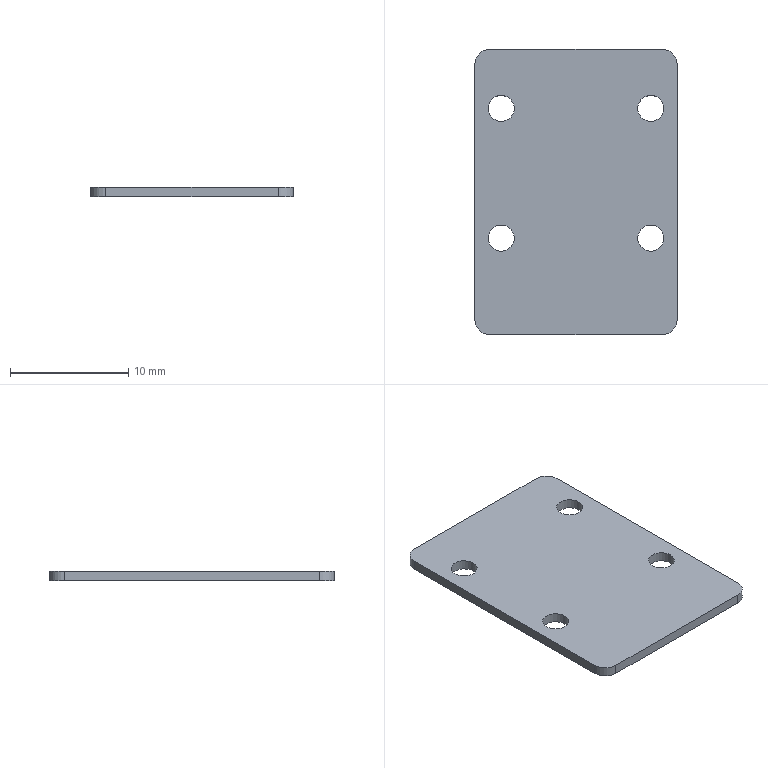Part | STEP file | VSWR protection V+PCB | 1 solid | 14 faces | box 17.08 x 24.07 x 0.832 mm | volume 328.245 mm3 | cylinder 8 | plane 6 | commonest cylinder face diameters 2.2 x4 2.54 x4
STEP:
#1=CARTESIAN_POINT('',(0.,0.,0.));
#2=DIRECTION('',(0.,0.,1.));
#3=DIRECTION('',(1.,0.,0.));
#4=AXIS2_PLACEMENT_3D('',#1,#2,#3);
#5=CARTESIAN_POINT('',(74.34,77.234,-0.832));
#6=VERTEX_POINT('',#5);
#7=CARTESIAN_POINT('',(73.24,77.234,-0.832));
#8=DIRECTION('',(0.,0.,1.));
#9=DIRECTION('',(1.,0.,0.));
#10=AXIS2_PLACEMENT_3D('',#7,#8,#9);
#11=CIRCLE('',#10,1.1);
#12=CARTESIAN_POINT('',(72.28,70.364,-0.832));
#13=DIRECTION('',(0.,0.,1.));
#14=DIRECTION('',(1.,0.,0.));
#15=AXIS2_PLACEMENT_3D('',#12,#13,#14);
#16=PLANE('',#15);
#17=CARTESIAN_POINT('',(0.96,6.87));
#18=DIRECTION('',(1.,0.));
#19=AXIS2_PLACEMENT_2D('',#17,#18);
#20=CIRCLE('',#19,1.1);
#21=(GEOMETRIC_REPRESENTATION_CONTEXT(2)PARAMETRIC_REPRESENTATION_CONTEXT()REPRESENTATION_CONTEXT('',''));
#22=DEFINITIONAL_REPRESENTATION('',(#20),#21);
#23=PCURVE('',#16,#22);
#24=CARTESIAN_POINT('',(73.24,77.234,-0.832));
#25=DIRECTION('',(0.,0.,1.));
#26=DIRECTION('',(1.,0.,0.));
#27=AXIS2_PLACEMENT_3D('',#24,#25,#26);
#28=CYLINDRICAL_SURFACE('',#27,1.1);
#29=CARTESIAN_POINT('',(0.,0.));
#30=DIRECTION('',(1.,0.));
#31=VECTOR('',#30,1.);
#32=LINE('',#29,#31);
#33=(GEOMETRIC_REPRESENTATION_CONTEXT(2)PARAMETRIC_REPRESENTATION_CONTEXT()REPRESENTATION_CONTEXT('',''));
#34=DEFINITIONAL_REPRESENTATION('',(#32),#33);
#35=PCURVE('',#28,#34);
#36=SURFACE_CURVE('',#11,(#23,#35),.PCURVE_S1.);
#37=EDGE_CURVE('',#6,#6,#36,.T.);
#38=ORIENTED_EDGE('',*,*,#37,.T.);
#39=EDGE_LOOP('',(#38));
#40=FACE_BOUND('',#39,.T.);
#41=CARTESIAN_POINT('',(86.96,77.234,-0.832));
#42=VERTEX_POINT('',#41);
#43=CARTESIAN_POINT('',(85.86,77.234,-0.832));
#44=DIRECTION('',(0.,0.,1.));
#45=DIRECTION('',(1.,0.,0.));
#46=AXIS2_PLACEMENT_3D('',#43,#44,#45);
#47=CIRCLE('',#46,1.1);
#48=CARTESIAN_POINT('',(13.58,6.87));
#49=DIRECTION('',(1.,0.));
#50=AXIS2_PLACEMENT_2D('',#48,#49);
#51=CIRCLE('',#50,1.1);
#52=(GEOMETRIC_REPRESENTATION_CONTEXT(2)PARAMETRIC_REPRESENTATION_CONTEXT()REPRESENTATION_CONTEXT('',''));
#53=DEFINITIONAL_REPRESENTATION('',(#51),#52);
#54=PCURVE('',#16,#53);
#55=CARTESIAN_POINT('',(85.86,77.234,-0.832));
#56=DIRECTION('',(0.,0.,1.));
#57=DIRECTION('',(1.,0.,0.));
#58=AXIS2_PLACEMENT_3D('',#55,#56,#57);
#59=CYLINDRICAL_SURFACE('',#58,1.1);
#60=CARTESIAN_POINT('',(0.,0.));
#61=DIRECTION('',(1.,0.));
#62=VECTOR('',#61,1.);
#63=LINE('',#60,#62);
#64=(GEOMETRIC_REPRESENTATION_CONTEXT(2)PARAMETRIC_REPRESENTATION_CONTEXT()REPRESENTATION_CONTEXT('',''));
#65=DEFINITIONAL_REPRESENTATION('',(#63),#64);
#66=PCURVE('',#59,#65);
#67=SURFACE_CURVE('',#47,(#54,#66),.PCURVE_S1.);
#68=EDGE_CURVE('',#42,#42,#67,.T.);
#69=ORIENTED_EDGE('',*,*,#68,.T.);
#70=EDGE_LOOP('',(#69));
#71=FACE_BOUND('',#70,.T.);
#72=CARTESIAN_POINT('',(86.96,88.184,-0.832));
#73=VERTEX_POINT('',#72);
#74=CARTESIAN_POINT('',(85.86,88.184,-0.832));
#75=DIRECTION('',(0.,0.,1.));
#76=DIRECTION('',(1.,0.,0.));
#77=AXIS2_PLACEMENT_3D('',#74,#75,#76);
#78=CIRCLE('',#77,1.1);
#79=CARTESIAN_POINT('',(13.58,17.82));
#80=DIRECTION('',(1.,0.));
#81=AXIS2_PLACEMENT_2D('',#79,#80);
#82=CIRCLE('',#81,1.1);
#83=(GEOMETRIC_REPRESENTATION_CONTEXT(2)PARAMETRIC_REPRESENTATION_CONTEXT()REPRESENTATION_CONTEXT('',''));
#84=DEFINITIONAL_REPRESENTATION('',(#82),#83);
#85=PCURVE('',#16,#84);
#86=CARTESIAN_POINT('',(85.86,88.184,-0.832));
#87=DIRECTION('',(0.,0.,1.));
#88=DIRECTION('',(1.,0.,0.));
#89=AXIS2_PLACEMENT_3D('',#86,#87,#88);
#90=CYLINDRICAL_SURFACE('',#89,1.1);
#91=CARTESIAN_POINT('',(0.,0.));
#92=DIRECTION('',(1.,0.));
#93=VECTOR('',#92,1.);
#94=LINE('',#91,#93);
#95=(GEOMETRIC_REPRESENTATION_CONTEXT(2)PARAMETRIC_REPRESENTATION_CONTEXT()REPRESENTATION_CONTEXT('',''));
#96=DEFINITIONAL_REPRESENTATION('',(#94),#95);
#97=PCURVE('',#90,#96);
#98=SURFACE_CURVE('',#78,(#85,#97),.PCURVE_S1.);
#99=EDGE_CURVE('',#73,#73,#98,.T.);
#100=ORIENTED_EDGE('',*,*,#99,.T.);
#101=EDGE_LOOP('',(#100));
#102=FACE_BOUND('',#101,.T.);
#103=CARTESIAN_POINT('',(71.01,91.894,-0.832));
#104=VERTEX_POINT('',#103);
#105=CARTESIAN_POINT('',(71.01,70.364,-0.832));
#106=VERTEX_POINT('',#105);
#107=CARTESIAN_POINT('',(71.01,91.894,-0.832));
#108=DIRECTION('',(0.,-1.,0.));
#109=VECTOR('',#108,1.);
#110=LINE('',#107,#109);
#111=CARTESIAN_POINT('',(-1.27,21.53));
#112=DIRECTION('',(0.,-1.));
#113=VECTOR('',#112,1.);
#114=LINE('',#111,#113);
#115=(GEOMETRIC_REPRESENTATION_CONTEXT(2)PARAMETRIC_REPRESENTATION_CONTEXT()REPRESENTATION_CONTEXT('',''));
#116=DEFINITIONAL_REPRESENTATION('',(#114),#115);
#117=PCURVE('',#16,#116);
#118=CARTESIAN_POINT('',(71.01,91.894,-0.832));
#119=DIRECTION('',(-1.,0.,0.));
#120=DIRECTION('',(0.,0.,1.));
#121=AXIS2_PLACEMENT_3D('',#118,#119,#120);
#122=PLANE('',#121);
#123=CARTESIAN_POINT('',(0.,0.));
#124=DIRECTION('',(0.,-1.));
#125=VECTOR('',#124,1.);
#126=LINE('',#123,#125);
#127=(GEOMETRIC_REPRESENTATION_CONTEXT(2)PARAMETRIC_REPRESENTATION_CONTEXT()REPRESENTATION_CONTEXT('',''));
#128=DEFINITIONAL_REPRESENTATION('',(#126),#127);
#129=PCURVE('',#122,#128);
#130=SURFACE_CURVE('',#110,(#117,#129),.PCURVE_S1.);
#131=EDGE_CURVE('',#104,#106,#130,.T.);
#132=ORIENTED_EDGE('',*,*,#131,.F.);
#133=CARTESIAN_POINT('',(72.28,93.164,-0.832));
#134=VERTEX_POINT('',#133);
#135=CARTESIAN_POINT('',(72.28,91.894,-0.832));
#136=DIRECTION('',(0.,0.,1.));
#137=DIRECTION('',(1.,0.,0.));
#138=AXIS2_PLACEMENT_3D('',#135,#136,#137);
#139=CIRCLE('',#138,1.27);
#140=CARTESIAN_POINT('',(0.,21.53));
#141=DIRECTION('',(1.,0.));
#142=AXIS2_PLACEMENT_2D('',#140,#141);
#143=CIRCLE('',#142,1.27);
#144=(GEOMETRIC_REPRESENTATION_CONTEXT(2)PARAMETRIC_REPRESENTATION_CONTEXT()REPRESENTATION_CONTEXT('',''));
#145=DEFINITIONAL_REPRESENTATION('',(#143),#144);
#146=PCURVE('',#16,#145);
#147=CARTESIAN_POINT('',(72.28,91.894,-0.832));
#148=DIRECTION('',(0.,0.,1.));
#149=DIRECTION('',(1.,0.,0.));
#150=AXIS2_PLACEMENT_3D('',#147,#148,#149);
#151=CYLINDRICAL_SURFACE('',#150,1.27);
#152=CARTESIAN_POINT('',(0.,0.));
#153=DIRECTION('',(1.,0.));
#154=VECTOR('',#153,1.);
#155=LINE('',#152,#154);
#156=(GEOMETRIC_REPRESENTATION_CONTEXT(2)PARAMETRIC_REPRESENTATION_CONTEXT()REPRESENTATION_CONTEXT('',''));
#157=DEFINITIONAL_REPRESENTATION('',(#155),#156);
#158=PCURVE('',#151,#157);
#159=SURFACE_CURVE('',#139,(#146,#158),.PCURVE_S1.);
#160=EDGE_CURVE('',#134,#104,#159,.T.);
#161=ORIENTED_EDGE('',*,*,#160,.F.);
#162=CARTESIAN_POINT('',(86.82,93.164,-0.832));
#163=VERTEX_POINT('',#162);
#164=CARTESIAN_POINT('',(86.82,93.164,-0.832));
#165=DIRECTION('',(-1.,0.,0.));
#166=VECTOR('',#165,1.);
#167=LINE('',#164,#166);
#168=CARTESIAN_POINT('',(14.54,22.8));
#169=DIRECTION('',(-1.,0.));
#170=VECTOR('',#169,1.);
#171=LINE('',#168,#170);
#172=(GEOMETRIC_REPRESENTATION_CONTEXT(2)PARAMETRIC_REPRESENTATION_CONTEXT()REPRESENTATION_CONTEXT('',''));
#173=DEFINITIONAL_REPRESENTATION('',(#171),#172);
#174=PCURVE('',#16,#173);
#175=CARTESIAN_POINT('',(79.55,93.164,-0.832));
#176=DIRECTION('',(0.,1.,0.));
#177=DIRECTION('',(0.,0.,1.));
#178=AXIS2_PLACEMENT_3D('',#175,#176,#177);
#179=PLANE('',#178);
#180=CARTESIAN_POINT('',(0.,7.27));
#181=DIRECTION('',(0.,-1.));
#182=VECTOR('',#181,1.);
#183=LINE('',#180,#182);
#184=(GEOMETRIC_REPRESENTATION_CONTEXT(2)PARAMETRIC_REPRESENTATION_CONTEXT()REPRESENTATION_CONTEXT('',''));
#185=DEFINITIONAL_REPRESENTATION('',(#183),#184);
#186=PCURVE('',#179,#185);
#187=SURFACE_CURVE('',#167,(#174,#186),.PCURVE_S1.);
#188=EDGE_CURVE('',#163,#134,#187,.T.);
#189=ORIENTED_EDGE('',*,*,#188,.F.);
#190=CARTESIAN_POINT('',(88.09,91.894,-0.832));
#191=VERTEX_POINT('',#190);
#192=CARTESIAN_POINT('',(86.82,91.894,-0.832));
#193=DIRECTION('',(0.,0.,1.));
#194=DIRECTION('',(1.,0.,0.));
#195=AXIS2_PLACEMENT_3D('',#192,#193,#194);
#196=CIRCLE('',#195,1.27);
#197=CARTESIAN_POINT('',(14.54,21.53));
#198=DIRECTION('',(1.,0.));
#199=AXIS2_PLACEMENT_2D('',#197,#198);
#200=CIRCLE('',#199,1.27);
#201=(GEOMETRIC_REPRESENTATION_CONTEXT(2)PARAMETRIC_REPRESENTATION_CONTEXT()REPRESENTATION_CONTEXT('',''));
#202=DEFINITIONAL_REPRESENTATION('',(#200),#201);
#203=PCURVE('',#16,#202);
#204=CARTESIAN_POINT('',(86.82,91.894,-0.832));
#205=DIRECTION('',(0.,0.,1.));
#206=DIRECTION('',(1.,0.,0.));
#207=AXIS2_PLACEMENT_3D('',#204,#205,#206);
#208=CYLINDRICAL_SURFACE('',#207,1.27);
#209=CARTESIAN_POINT('',(0.,0.));
#210=DIRECTION('',(1.,0.));
#211=VECTOR('',#210,1.);
#212=LINE('',#209,#211);
#213=(GEOMETRIC_REPRESENTATION_CONTEXT(2)PARAMETRIC_REPRESENTATION_CONTEXT()REPRESENTATION_CONTEXT('',''));
#214=DEFINITIONAL_REPRESENTATION('',(#212),#213);
#215=PCURVE('',#208,#214);
#216=SURFACE_CURVE('',#196,(#203,#215),.PCURVE_S1.);
#217=EDGE_CURVE('',#191,#163,#216,.T.);
#218=ORIENTED_EDGE('',*,*,#217,.F.);
#219=CARTESIAN_POINT('',(88.09,70.364,-0.832));
#220=VERTEX_POINT('',#219);
#221=CARTESIAN_POINT('',(88.09,70.364,-0.832));
#222=DIRECTION('',(0.,1.,0.));
#223=VECTOR('',#222,1.);
#224=LINE('',#221,#223);
#225=CARTESIAN_POINT('',(15.81,0.));
#226=DIRECTION('',(0.,1.));
#227=VECTOR('',#226,1.);
#228=LINE('',#225,#227);
#229=(GEOMETRIC_REPRESENTATION_CONTEXT(2)PARAMETRIC_REPRESENTATION_CONTEXT()REPRESENTATION_CONTEXT('',''));
#230=DEFINITIONAL_REPRESENTATION('',(#228),#229);
#231=PCURVE('',#16,#230);
#232=CARTESIAN_POINT('',(88.09,70.364,-0.832));
#233=DIRECTION('',(1.,0.,0.));
#234=DIRECTION('',(0.,0.,-1.));
#235=AXIS2_PLACEMENT_3D('',#232,#233,#234);
#236=PLANE('',#235);
#237=CARTESIAN_POINT('',(0.,0.));
#238=DIRECTION('',(0.,1.));
#239=VECTOR('',#238,1.);
#240=LINE('',#237,#239);
#241=(GEOMETRIC_REPRESENTATION_CONTEXT(2)PARAMETRIC_REPRESENTATION_CONTEXT()REPRESENTATION_CONTEXT('',''));
#242=DEFINITIONAL_REPRESENTATION('',(#240),#241);
#243=PCURVE('',#236,#242);
#244=SURFACE_CURVE('',#224,(#231,#243),.PCURVE_S1.);
#245=EDGE_CURVE('',#220,#191,#244,.T.);
#246=ORIENTED_EDGE('',*,*,#245,.F.);
#247=CARTESIAN_POINT('',(86.82,69.094,-0.832));
#248=VERTEX_POINT('',#247);
#249=CARTESIAN_POINT('',(86.82,70.364,-0.832));
#250=DIRECTION('',(0.,0.,1.));
#251=DIRECTION('',(1.,0.,0.));
#252=AXIS2_PLACEMENT_3D('',#249,#250,#251);
#253=CIRCLE('',#252,1.27);
#254=CARTESIAN_POINT('',(14.54,0.));
#255=DIRECTION('',(1.,0.));
#256=AXIS2_PLACEMENT_2D('',#254,#255);
#257=CIRCLE('',#256,1.27);
#258=(GEOMETRIC_REPRESENTATION_CONTEXT(2)PARAMETRIC_REPRESENTATION_CONTEXT()REPRESENTATION_CONTEXT('',''));
#259=DEFINITIONAL_REPRESENTATION('',(#257),#258);
#260=PCURVE('',#16,#259);
#261=CARTESIAN_POINT('',(86.82,70.364,-0.832));
#262=DIRECTION('',(0.,0.,1.));
#263=DIRECTION('',(1.,0.,0.));
#264=AXIS2_PLACEMENT_3D('',#261,#262,#263);
#265=CYLINDRICAL_SURFACE('',#264,1.27);
#266=CARTESIAN_POINT('',(0.,0.));
#267=DIRECTION('',(1.,0.));
#268=VECTOR('',#267,1.);
#269=LINE('',#266,#268);
#270=(GEOMETRIC_REPRESENTATION_CONTEXT(2)PARAMETRIC_REPRESENTATION_CONTEXT()REPRESENTATION_CONTEXT('',''));
#271=DEFINITIONAL_REPRESENTATION('',(#269),#270);
#272=PCURVE('',#265,#271);
#273=SURFACE_CURVE('',#253,(#260,#272),.PCURVE_S1.);
#274=EDGE_CURVE('',#248,#220,#273,.T.);
#275=ORIENTED_EDGE('',*,*,#274,.F.);
#276=CARTESIAN_POINT('',(72.28,69.094,-0.832));
#277=VERTEX_POINT('',#276);
#278=CARTESIAN_POINT('',(72.28,69.094,-0.832));
#279=DIRECTION('',(1.,0.,0.));
#280=VECTOR('',#279,1.);
#281=LINE('',#278,#280);
#282=CARTESIAN_POINT('',(0.,-1.27));
#283=DIRECTION('',(1.,0.));
#284=VECTOR('',#283,1.);
#285=LINE('',#282,#284);
#286=(GEOMETRIC_REPRESENTATION_CONTEXT(2)PARAMETRIC_REPRESENTATION_CONTEXT()REPRESENTATION_CONTEXT('',''));
#287=DEFINITIONAL_REPRESENTATION('',(#285),#286);
#288=PCURVE('',#16,#287);
#289=CARTESIAN_POINT('',(72.28,69.094,-0.832));
#290=DIRECTION('',(0.,-1.,0.));
#291=DIRECTION('',(0.,0.,-1.));
#292=AXIS2_PLACEMENT_3D('',#289,#290,#291);
#293=PLANE('',#292);
#294=CARTESIAN_POINT('',(0.,0.));
#295=DIRECTION('',(0.,1.));
#296=VECTOR('',#295,1.);
#297=LINE('',#294,#296);
#298=(GEOMETRIC_REPRESENTATION_CONTEXT(2)PARAMETRIC_REPRESENTATION_CONTEXT()REPRESENTATION_CONTEXT('',''));
#299=DEFINITIONAL_REPRESENTATION('',(#297),#298);
#300=PCURVE('',#293,#299);
#301=SURFACE_CURVE('',#281,(#288,#300),.PCURVE_S1.);
#302=EDGE_CURVE('',#277,#248,#301,.T.);
#303=ORIENTED_EDGE('',*,*,#302,.F.);
#304=CARTESIAN_POINT('',(72.28,70.364,-0.832));
#305=DIRECTION('',(0.,0.,1.));
#306=DIRECTION('',(1.,0.,0.));
#307=AXIS2_PLACEMENT_3D('',#304,#305,#306);
#308=CIRCLE('',#307,1.27);
#309=CARTESIAN_POINT('',(0.,0.));
#310=DIRECTION('',(1.,0.));
#311=AXIS2_PLACEMENT_2D('',#309,#310);
#312=CIRCLE('',#311,1.27);
#313=(GEOMETRIC_REPRESENTATION_CONTEXT(2)PARAMETRIC_REPRESENTATION_CONTEXT()REPRESENTATION_CONTEXT('',''));
#314=DEFINITIONAL_REPRESENTATION('',(#312),#313);
#315=PCURVE('',#16,#314);
#316=CARTESIAN_POINT('',(72.28,70.364,-0.832));
#317=DIRECTION('',(0.,0.,1.));
#318=DIRECTION('',(1.,0.,0.));
#319=AXIS2_PLACEMENT_3D('',#316,#317,#318);
#320=CYLINDRICAL_SURFACE('',#319,1.27);
#321=CARTESIAN_POINT('',(0.,0.));
#322=DIRECTION('',(1.,0.));
#323=VECTOR('',#322,1.);
#324=LINE('',#321,#323);
#325=(GEOMETRIC_REPRESENTATION_CONTEXT(2)PARAMETRIC_REPRESENTATION_CONTEXT()REPRESENTATION_CONTEXT('',''));
#326=DEFINITIONAL_REPRESENTATION('',(#324),#325);
#327=PCURVE('',#320,#326);
#328=SURFACE_CURVE('',#308,(#315,#327),.PCURVE_S1.);
#329=EDGE_CURVE('',#106,#277,#328,.T.);
#330=ORIENTED_EDGE('',*,*,#329,.F.);
#331=EDGE_LOOP('',(#132,#161,#189,#218,#246,#275,#303,#330));
#332=FACE_BOUND('',#331,.T.);
#333=CARTESIAN_POINT('',(74.34,88.184,-0.832));
#334=VERTEX_POINT('',#333);
#335=CARTESIAN_POINT('',(73.24,88.184,-0.832));
#336=DIRECTION('',(0.,0.,-1.));
#337=DIRECTION('',(1.,0.,0.));
#338=AXIS2_PLACEMENT_3D('',#335,#336,#337);
#339=CIRCLE('',#338,1.1);
#340=CARTESIAN_POINT('',(2.06,17.82));
#341=CARTESIAN_POINT('',(2.06,15.915));
#342=CARTESIAN_POINT('',(0.41,16.867));
#343=CARTESIAN_POINT('',(-1.24,17.82));
#344=CARTESIAN_POINT('',(0.41,18.773));
#345=CARTESIAN_POINT('',(2.06,19.725));
#346=CARTESIAN_POINT('',(2.06,17.82));
#347=(BOUNDED_CURVE()B_SPLINE_CURVE(2,(#340,#341,#342,#343,#344,#345,#346),.UNSPECIFIED.,.T.,.F.)B_SPLINE_CURVE_WITH_KNOTS((1,2,2,2,2,1),(-2.094,0.,2.094,4.189,6.283,8.378),.UNSPECIFIED.)CURVE()GEOMETRIC_REPRESENTATION_ITEM()RATIONAL_B_SPLINE_CURVE((1.,0.5,1.,0.5,1.,0.5,1.))REPRESENTATION_ITEM(''));
#348=(GEOMETRIC_REPRESENTATION_CONTEXT(2)PARAMETRIC_REPRESENTATION_CONTEXT()REPRESENTATION_CONTEXT('',''));
#349=DEFINITIONAL_REPRESENTATION('',(#347),#348);
#350=PCURVE('',#16,#349);
#351=CARTESIAN_POINT('',(73.24,88.184,-0.832));
#352=DIRECTION('',(0.,0.,1.));
#353=DIRECTION('',(1.,0.,0.));
#354=AXIS2_PLACEMENT_3D('',#351,#352,#353);
#355=CYLINDRICAL_SURFACE('',#354,1.1);
#356=CARTESIAN_POINT('',(6.283,0.));
#357=DIRECTION('',(-1.,0.));
#358=VECTOR('',#357,1.);
#359=LINE('',#356,#358);
#360=(GEOMETRIC_REPRESENTATION_CONTEXT(2)PARAMETRIC_REPRESENTATION_CONTEXT()REPRESENTATION_CONTEXT('',''));
#361=DEFINITIONAL_REPRESENTATION('',(#359),#360);
#362=PCURVE('',#355,#361);
#363=SURFACE_CURVE('',#339,(#350,#362),.PCURVE_S1.);
#364=EDGE_CURVE('',#334,#334,#363,.T.);
#365=ORIENTED_EDGE('',*,*,#364,.F.);
#366=EDGE_LOOP('',(#365));
#367=FACE_BOUND('',#366,.T.);
#368=ADVANCED_FACE('',(#40,#71,#102,#332,#367),#16,.F.);
#369=CARTESIAN_POINT('',(71.01,91.894,0.));
#370=VERTEX_POINT('',#369);
#371=CARTESIAN_POINT('',(71.01,70.364,0.));
#372=VERTEX_POINT('',#371);
#373=CARTESIAN_POINT('',(71.01,91.894,0.));
#374=DIRECTION('',(0.,-1.,0.));
#375=VECTOR('',#374,1.);
#376=LINE('',#373,#375);
#377=CARTESIAN_POINT('',(72.28,70.364,0.));
#378=DIRECTION('',(0.,0.,1.));
#379=DIRECTION('',(1.,0.,0.));
#380=AXIS2_PLACEMENT_3D('',#377,#378,#379);
#381=PLANE('',#380);
#382=CARTESIAN_POINT('',(-1.27,21.53));
#383=DIRECTION('',(0.,-1.));
#384=VECTOR('',#383,1.);
#385=LINE('',#382,#384);
#386=(GEOMETRIC_REPRESENTATION_CONTEXT(2)PARAMETRIC_REPRESENTATION_CONTEXT()REPRESENTATION_CONTEXT('',''));
#387=DEFINITIONAL_REPRESENTATION('',(#385),#386);
#388=PCURVE('',#381,#387);
#389=CARTESIAN_POINT('',(0.832,0.));
#390=DIRECTION('',(0.,-1.));
#391=VECTOR('',#390,1.);
#392=LINE('',#389,#391);
#393=(GEOMETRIC_REPRESENTATION_CONTEXT(2)PARAMETRIC_REPRESENTATION_CONTEXT()REPRESENTATION_CONTEXT('',''));
#394=DEFINITIONAL_REPRESENTATION('',(#392),#393);
#395=PCURVE('',#122,#394);
#396=SURFACE_CURVE('',#376,(#388,#395),.PCURVE_S1.);
#397=EDGE_CURVE('',#370,#372,#396,.T.);
#398=ORIENTED_EDGE('',*,*,#397,.T.);
#399=CARTESIAN_POINT('',(72.28,69.094,0.));
#400=VERTEX_POINT('',#399);
#401=CARTESIAN_POINT('',(72.28,70.364,0.));
#402=DIRECTION('',(0.,0.,1.));
#403=DIRECTION('',(1.,0.,0.));
#404=AXIS2_PLACEMENT_3D('',#401,#402,#403);
#405=CIRCLE('',#404,1.27);
#406=CARTESIAN_POINT('',(0.,0.));
#407=DIRECTION('',(1.,0.));
#408=AXIS2_PLACEMENT_2D('',#406,#407);
#409=CIRCLE('',#408,1.27);
#410=(GEOMETRIC_REPRESENTATION_CONTEXT(2)PARAMETRIC_REPRESENTATION_CONTEXT()REPRESENTATION_CONTEXT('',''));
#411=DEFINITIONAL_REPRESENTATION('',(#409),#410);
#412=PCURVE('',#381,#411);
#413=CARTESIAN_POINT('',(0.,0.832));
#414=DIRECTION('',(1.,0.));
#415=VECTOR('',#414,1.);
#416=LINE('',#413,#415);
#417=(GEOMETRIC_REPRESENTATION_CONTEXT(2)PARAMETRIC_REPRESENTATION_CONTEXT()REPRESENTATION_CONTEXT('',''));
#418=DEFINITIONAL_REPRESENTATION('',(#416),#417);
#419=PCURVE('',#320,#418);
#420=SURFACE_CURVE('',#405,(#412,#419),.PCURVE_S1.);
#421=EDGE_CURVE('',#372,#400,#420,.T.);
#422=ORIENTED_EDGE('',*,*,#421,.T.);
#423=CARTESIAN_POINT('',(86.82,69.094,0.));
#424=VERTEX_POINT('',#423);
#425=CARTESIAN_POINT('',(72.28,69.094,0.));
#426=DIRECTION('',(1.,0.,0.));
#427=VECTOR('',#426,1.);
#428=LINE('',#425,#427);
#429=CARTESIAN_POINT('',(0.,-1.27));
#430=DIRECTION('',(1.,0.));
#431=VECTOR('',#430,1.);
#432=LINE('',#429,#431);
#433=(GEOMETRIC_REPRESENTATION_CONTEXT(2)PARAMETRIC_REPRESENTATION_CONTEXT()REPRESENTATION_CONTEXT('',''));
#434=DEFINITIONAL_REPRESENTATION('',(#432),#433);
#435=PCURVE('',#381,#434);
#436=CARTESIAN_POINT('',(-0.832,0.));
#437=DIRECTION('',(0.,1.));
#438=VECTOR('',#437,1.);
#439=LINE('',#436,#438);
#440=(GEOMETRIC_REPRESENTATION_CONTEXT(2)PARAMETRIC_REPRESENTATION_CONTEXT()REPRESENTATION_CONTEXT('',''));
#441=DEFINITIONAL_REPRESENTATION('',(#439),#440);
#442=PCURVE('',#293,#441);
#443=SURFACE_CURVE('',#428,(#435,#442),.PCURVE_S1.);
#444=EDGE_CURVE('',#400,#424,#443,.T.);
#445=ORIENTED_EDGE('',*,*,#444,.T.);
#446=CARTESIAN_POINT('',(88.09,70.364,0.));
#447=VERTEX_POINT('',#446);
#448=CARTESIAN_POINT('',(86.82,70.364,0.));
#449=DIRECTION('',(0.,0.,1.));
#450=DIRECTION('',(1.,0.,0.));
#451=AXIS2_PLACEMENT_3D('',#448,#449,#450);
#452=CIRCLE('',#451,1.27);
#453=CARTESIAN_POINT('',(14.54,0.));
#454=DIRECTION('',(1.,0.));
#455=AXIS2_PLACEMENT_2D('',#453,#454);
#456=CIRCLE('',#455,1.27);
#457=(GEOMETRIC_REPRESENTATION_CONTEXT(2)PARAMETRIC_REPRESENTATION_CONTEXT()REPRESENTATION_CONTEXT('',''));
#458=DEFINITIONAL_REPRESENTATION('',(#456),#457);
#459=PCURVE('',#381,#458);
#460=CARTESIAN_POINT('',(0.,0.832));
#461=DIRECTION('',(1.,0.));
#462=VECTOR('',#461,1.);
#463=LINE('',#460,#462);
#464=(GEOMETRIC_REPRESENTATION_CONTEXT(2)PARAMETRIC_REPRESENTATION_CONTEXT()REPRESENTATION_CONTEXT('',''));
#465=DEFINITIONAL_REPRESENTATION('',(#463),#464);
#466=PCURVE('',#265,#465);
#467=SURFACE_CURVE('',#452,(#459,#466),.PCURVE_S1.);
#468=EDGE_CURVE('',#424,#447,#467,.T.);
#469=ORIENTED_EDGE('',*,*,#468,.T.);
#470=CARTESIAN_POINT('',(88.09,91.894,0.));
#471=VERTEX_POINT('',#470);
#472=CARTESIAN_POINT('',(88.09,70.364,0.));
#473=DIRECTION('',(0.,1.,0.));
#474=VECTOR('',#473,1.);
#475=LINE('',#472,#474);
#476=CARTESIAN_POINT('',(15.81,0.));
#477=DIRECTION('',(0.,1.));
#478=VECTOR('',#477,1.);
#479=LINE('',#476,#478);
#480=(GEOMETRIC_REPRESENTATION_CONTEXT(2)PARAMETRIC_REPRESENTATION_CONTEXT()REPRESENTATION_CONTEXT('',''));
#481=DEFINITIONAL_REPRESENTATION('',(#479),#480);
#482=PCURVE('',#381,#481);
#483=CARTESIAN_POINT('',(-0.832,0.));
#484=DIRECTION('',(0.,1.));
#485=VECTOR('',#484,1.);
#486=LINE('',#483,#485);
#487=(GEOMETRIC_REPRESENTATION_CONTEXT(2)PARAMETRIC_REPRESENTATION_CONTEXT()REPRESENTATION_CONTEXT('',''));
#488=DEFINITIONAL_REPRESENTATION('',(#486),#487);
#489=PCURVE('',#236,#488);
#490=SURFACE_CURVE('',#475,(#482,#489),.PCURVE_S1.);
#491=EDGE_CURVE('',#447,#471,#490,.T.);
#492=ORIENTED_EDGE('',*,*,#491,.T.);
#493=CARTESIAN_POINT('',(86.82,93.164,0.));
#494=VERTEX_POINT('',#493);
#495=CARTESIAN_POINT('',(86.82,91.894,0.));
#496=DIRECTION('',(0.,0.,1.));
#497=DIRECTION('',(1.,0.,0.));
#498=AXIS2_PLACEMENT_3D('',#495,#496,#497);
#499=CIRCLE('',#498,1.27);
#500=CARTESIAN_POINT('',(14.54,21.53));
#501=DIRECTION('',(1.,0.));
#502=AXIS2_PLACEMENT_2D('',#500,#501);
#503=CIRCLE('',#502,1.27);
#504=(GEOMETRIC_REPRESENTATION_CONTEXT(2)PARAMETRIC_REPRESENTATION_CONTEXT()REPRESENTATION_CONTEXT('',''));
#505=DEFINITIONAL_REPRESENTATION('',(#503),#504);
#506=PCURVE('',#381,#505);
#507=CARTESIAN_POINT('',(0.,0.832));
#508=DIRECTION('',(1.,0.));
#509=VECTOR('',#508,1.);
#510=LINE('',#507,#509);
#511=(GEOMETRIC_REPRESENTATION_CONTEXT(2)PARAMETRIC_REPRESENTATION_CONTEXT()REPRESENTATION_CONTEXT('',''));
#512=DEFINITIONAL_REPRESENTATION('',(#510),#511);
#513=PCURVE('',#208,#512);
#514=SURFACE_CURVE('',#499,(#506,#513),.PCURVE_S1.);
#515=EDGE_CURVE('',#471,#494,#514,.T.);
#516=ORIENTED_EDGE('',*,*,#515,.T.);
#517=CARTESIAN_POINT('',(72.28,93.164,0.));
#518=VERTEX_POINT('',#517);
#519=CARTESIAN_POINT('',(79.55,93.164,0.));
#520=DIRECTION('',(-1.,0.,0.));
#521=VECTOR('',#520,1.);
#522=LINE('',#519,#521);
#523=CARTESIAN_POINT('',(7.27,22.8));
#524=DIRECTION('',(-1.,0.));
#525=VECTOR('',#524,1.);
#526=LINE('',#523,#525);
#527=(GEOMETRIC_REPRESENTATION_CONTEXT(2)PARAMETRIC_REPRESENTATION_CONTEXT()REPRESENTATION_CONTEXT('',''));
#528=DEFINITIONAL_REPRESENTATION('',(#526),#527);
#529=PCURVE('',#381,#528);
#530=CARTESIAN_POINT('',(0.832,0.));
#531=DIRECTION('',(0.,-1.));
#532=VECTOR('',#531,1.);
#533=LINE('',#530,#532);
#534=(GEOMETRIC_REPRESENTATION_CONTEXT(2)PARAMETRIC_REPRESENTATION_CONTEXT()REPRESENTATION_CONTEXT('',''));
#535=DEFINITIONAL_REPRESENTATION('',(#533),#534);
#536=PCURVE('',#179,#535);
#537=SURFACE_CURVE('',#522,(#529,#536),.PCURVE_S1.);
#538=EDGE_CURVE('',#494,#518,#537,.T.);
#539=ORIENTED_EDGE('',*,*,#538,.T.);
#540=CARTESIAN_POINT('',(72.28,91.894,0.));
#541=DIRECTION('',(0.,0.,1.));
#542=DIRECTION('',(1.,0.,0.));
#543=AXIS2_PLACEMENT_3D('',#540,#541,#542);
#544=CIRCLE('',#543,1.27);
#545=CARTESIAN_POINT('',(0.,21.53));
#546=DIRECTION('',(1.,0.));
#547=AXIS2_PLACEMENT_2D('',#545,#546);
#548=CIRCLE('',#547,1.27);
#549=(GEOMETRIC_REPRESENTATION_CONTEXT(2)PARAMETRIC_REPRESENTATION_CONTEXT()REPRESENTATION_CONTEXT('',''));
#550=DEFINITIONAL_REPRESENTATION('',(#548),#549);
#551=PCURVE('',#381,#550);
#552=CARTESIAN_POINT('',(0.,0.832));
#553=DIRECTION('',(1.,0.));
#554=VECTOR('',#553,1.);
#555=LINE('',#552,#554);
#556=(GEOMETRIC_REPRESENTATION_CONTEXT(2)PARAMETRIC_REPRESENTATION_CONTEXT()REPRESENTATION_CONTEXT('',''));
#557=DEFINITIONAL_REPRESENTATION('',(#555),#556);
#558=PCURVE('',#151,#557);
#559=SURFACE_CURVE('',#544,(#551,#558),.PCURVE_S1.);
#560=EDGE_CURVE('',#518,#370,#559,.T.);
#561=ORIENTED_EDGE('',*,*,#560,.T.);
#562=EDGE_LOOP('',(#398,#422,#445,#469,#492,#516,#539,#561));
#563=FACE_BOUND('',#562,.T.);
#564=CARTESIAN_POINT('',(86.96,88.184,0.));
#565=VERTEX_POINT('',#564);
#566=CARTESIAN_POINT('',(85.86,88.184,0.));
#567=DIRECTION('',(0.,0.,1.));
#568=DIRECTION('',(1.,0.,0.));
#569=AXIS2_PLACEMENT_3D('',#566,#567,#568);
#570=CIRCLE('',#569,1.1);
#571=CARTESIAN_POINT('',(13.58,17.82));
#572=DIRECTION('',(1.,0.));
#573=AXIS2_PLACEMENT_2D('',#571,#572);
#574=CIRCLE('',#573,1.1);
#575=(GEOMETRIC_REPRESENTATION_CONTEXT(2)PARAMETRIC_REPRESENTATION_CONTEXT()REPRESENTATION_CONTEXT('',''));
#576=DEFINITIONAL_REPRESENTATION('',(#574),#575);
#577=PCURVE('',#381,#576);
#578=CARTESIAN_POINT('',(0.,0.832));
#579=DIRECTION('',(1.,0.));
#580=VECTOR('',#579,1.);
#581=LINE('',#578,#580);
#582=(GEOMETRIC_REPRESENTATION_CONTEXT(2)PARAMETRIC_REPRESENTATION_CONTEXT()REPRESENTATION_CONTEXT('',''));
#583=DEFINITIONAL_REPRESENTATION('',(#581),#582);
#584=PCURVE('',#90,#583);
#585=SURFACE_CURVE('',#570,(#577,#584),.PCURVE_S1.);
#586=EDGE_CURVE('',#565,#565,#585,.T.);
#587=ORIENTED_EDGE('',*,*,#586,.F.);
#588=EDGE_LOOP('',(#587));
#589=FACE_BOUND('',#588,.T.);
#590=CARTESIAN_POINT('',(86.96,77.234,0.));
#591=VERTEX_POINT('',#590);
#592=CARTESIAN_POINT('',(85.86,77.234,0.));
#593=DIRECTION('',(0.,0.,1.));
#594=DIRECTION('',(1.,0.,0.));
#595=AXIS2_PLACEMENT_3D('',#592,#593,#594);
#596=CIRCLE('',#595,1.1);
#597=CARTESIAN_POINT('',(13.58,6.87));
#598=DIRECTION('',(1.,0.));
#599=AXIS2_PLACEMENT_2D('',#597,#598);
#600=CIRCLE('',#599,1.1);
#601=(GEOMETRIC_REPRESENTATION_CONTEXT(2)PARAMETRIC_REPRESENTATION_CONTEXT()REPRESENTATION_CONTEXT('',''));
#602=DEFINITIONAL_REPRESENTATION('',(#600),#601);
#603=PCURVE('',#381,#602);
#604=CARTESIAN_POINT('',(0.,0.832));
#605=DIRECTION('',(1.,0.));
#606=VECTOR('',#605,1.);
#607=LINE('',#604,#606);
#608=(GEOMETRIC_REPRESENTATION_CONTEXT(2)PARAMETRIC_REPRESENTATION_CONTEXT()REPRESENTATION_CONTEXT('',''));
#609=DEFINITIONAL_REPRESENTATION('',(#607),#608);
#610=PCURVE('',#59,#609);
#611=SURFACE_CURVE('',#596,(#603,#610),.PCURVE_S1.);
#612=EDGE_CURVE('',#591,#591,#611,.T.);
#613=ORIENTED_EDGE('',*,*,#612,.F.);
#614=EDGE_LOOP('',(#613));
#615=FACE_BOUND('',#614,.T.);
#616=CARTESIAN_POINT('',(74.34,77.234,0.));
#617=VERTEX_POINT('',#616);
#618=CARTESIAN_POINT('',(73.24,77.234,0.));
#619=DIRECTION('',(0.,0.,1.));
#620=DIRECTION('',(1.,0.,0.));
#621=AXIS2_PLACEMENT_3D('',#618,#619,#620);
#622=CIRCLE('',#621,1.1);
#623=CARTESIAN_POINT('',(0.96,6.87));
#624=DIRECTION('',(1.,0.));
#625=AXIS2_PLACEMENT_2D('',#623,#624);
#626=CIRCLE('',#625,1.1);
#627=(GEOMETRIC_REPRESENTATION_CONTEXT(2)PARAMETRIC_REPRESENTATION_CONTEXT()REPRESENTATION_CONTEXT('',''));
#628=DEFINITIONAL_REPRESENTATION('',(#626),#627);
#629=PCURVE('',#381,#628);
#630=CARTESIAN_POINT('',(0.,0.832));
#631=DIRECTION('',(1.,0.));
#632=VECTOR('',#631,1.);
#633=LINE('',#630,#632);
#634=(GEOMETRIC_REPRESENTATION_CONTEXT(2)PARAMETRIC_REPRESENTATION_CONTEXT()REPRESENTATION_CONTEXT('',''));
#635=DEFINITIONAL_REPRESENTATION('',(#633),#634);
#636=PCURVE('',#28,#635);
#637=SURFACE_CURVE('',#622,(#629,#636),.PCURVE_S1.);
#638=EDGE_CURVE('',#617,#617,#637,.T.);
#639=ORIENTED_EDGE('',*,*,#638,.F.);
#640=EDGE_LOOP('',(#639));
#641=FACE_BOUND('',#640,.T.);
#642=CARTESIAN_POINT('',(74.34,88.184,0.));
#643=VERTEX_POINT('',#642);
#644=CARTESIAN_POINT('',(73.24,88.184,0.));
#645=DIRECTION('',(0.,0.,-1.));
#646=DIRECTION('',(1.,0.,0.));
#647=AXIS2_PLACEMENT_3D('',#644,#645,#646);
#648=CIRCLE('',#647,1.1);
#649=CARTESIAN_POINT('',(2.06,17.82));
#650=CARTESIAN_POINT('',(2.06,15.915));
#651=CARTESIAN_POINT('',(0.41,16.867));
#652=CARTESIAN_POINT('',(-1.24,17.82));
#653=CARTESIAN_POINT('',(0.41,18.773));
#654=CARTESIAN_POINT('',(2.06,19.725));
#655=CARTESIAN_POINT('',(2.06,17.82));
#656=(BOUNDED_CURVE()B_SPLINE_CURVE(2,(#649,#650,#651,#652,#653,#654,#655),.UNSPECIFIED.,.T.,.F.)B_SPLINE_CURVE_WITH_KNOTS((1,2,2,2,2,1),(-2.094,0.,2.094,4.189,6.283,8.378),.UNSPECIFIED.)CURVE()GEOMETRIC_REPRESENTATION_ITEM()RATIONAL_B_SPLINE_CURVE((1.,0.5,1.,0.5,1.,0.5,1.))REPRESENTATION_ITEM(''));
#657=(GEOMETRIC_REPRESENTATION_CONTEXT(2)PARAMETRIC_REPRESENTATION_CONTEXT()REPRESENTATION_CONTEXT('',''));
#658=DEFINITIONAL_REPRESENTATION('',(#656),#657);
#659=PCURVE('',#381,#658);
#660=CARTESIAN_POINT('',(6.283,0.832));
#661=DIRECTION('',(-1.,0.));
#662=VECTOR('',#661,1.);
#663=LINE('',#660,#662);
#664=(GEOMETRIC_REPRESENTATION_CONTEXT(2)PARAMETRIC_REPRESENTATION_CONTEXT()REPRESENTATION_CONTEXT('',''));
#665=DEFINITIONAL_REPRESENTATION('',(#663),#664);
#666=PCURVE('',#355,#665);
#667=SURFACE_CURVE('',#648,(#659,#666),.PCURVE_S1.);
#668=EDGE_CURVE('',#643,#643,#667,.T.);
#669=ORIENTED_EDGE('',*,*,#668,.T.);
#670=EDGE_LOOP('',(#669));
#671=FACE_BOUND('',#670,.T.);
#672=ADVANCED_FACE('',(#563,#589,#615,#641,#671),#381,.T.);
#673=ORIENTED_EDGE('',*,*,#397,.F.);
#674=CARTESIAN_POINT('',(71.01,91.894,-0.832));
#675=DIRECTION('',(0.,0.,1.));
#676=VECTOR('',#675,1.);
#677=LINE('',#674,#676);
#678=CARTESIAN_POINT('',(0.,0.));
#679=DIRECTION('',(1.,0.));
#680=VECTOR('',#679,1.);
#681=LINE('',#678,#680);
#682=(GEOMETRIC_REPRESENTATION_CONTEXT(2)PARAMETRIC_REPRESENTATION_CONTEXT()REPRESENTATION_CONTEXT('',''));
#683=DEFINITIONAL_REPRESENTATION('',(#681),#682);
#684=PCURVE('',#122,#683);
#685=CARTESIAN_POINT('',(3.142,0.));
#686=DIRECTION('',(0.,1.));
#687=VECTOR('',#686,1.);
#688=LINE('',#685,#687);
#689=(GEOMETRIC_REPRESENTATION_CONTEXT(2)PARAMETRIC_REPRESENTATION_CONTEXT()REPRESENTATION_CONTEXT('',''));
#690=DEFINITIONAL_REPRESENTATION('',(#688),#689);
#691=PCURVE('',#151,#690);
#692=SURFACE_CURVE('',#677,(#684,#691),.PCURVE_S1.);
#693=EDGE_CURVE('',#104,#370,#692,.T.);
#694=ORIENTED_EDGE('',*,*,#693,.F.);
#695=ORIENTED_EDGE('',*,*,#131,.T.);
#696=CARTESIAN_POINT('',(71.01,70.364,-0.832));
#697=DIRECTION('',(0.,0.,1.));
#698=VECTOR('',#697,1.);
#699=LINE('',#696,#698);
#700=CARTESIAN_POINT('',(0.,-21.53));
#701=DIRECTION('',(1.,0.));
#702=VECTOR('',#701,1.);
#703=LINE('',#700,#702);
#704=(GEOMETRIC_REPRESENTATION_CONTEXT(2)PARAMETRIC_REPRESENTATION_CONTEXT()REPRESENTATION_CONTEXT('',''));
#705=DEFINITIONAL_REPRESENTATION('',(#703),#704);
#706=PCURVE('',#122,#705);
#707=CARTESIAN_POINT('',(3.142,0.));
#708=DIRECTION('',(0.,1.));
#709=VECTOR('',#708,1.);
#710=LINE('',#707,#709);
#711=(GEOMETRIC_REPRESENTATION_CONTEXT(2)PARAMETRIC_REPRESENTATION_CONTEXT()REPRESENTATION_CONTEXT('',''));
#712=DEFINITIONAL_REPRESENTATION('',(#710),#711);
#713=PCURVE('',#320,#712);
#714=SURFACE_CURVE('',#699,(#706,#713),.PCURVE_S1.);
#715=EDGE_CURVE('',#106,#372,#714,.T.);
#716=ORIENTED_EDGE('',*,*,#715,.T.);
#717=EDGE_LOOP('',(#673,#694,#695,#716));
#718=FACE_BOUND('',#717,.T.);
#719=ADVANCED_FACE('',(#718),#122,.T.);
#720=ORIENTED_EDGE('',*,*,#421,.F.);
#721=ORIENTED_EDGE('',*,*,#715,.F.);
#722=ORIENTED_EDGE('',*,*,#329,.T.);
#723=CARTESIAN_POINT('',(72.28,69.094,-0.832));
#724=DIRECTION('',(0.,0.,1.));
#725=VECTOR('',#724,1.);
#726=LINE('',#723,#725);
#727=CARTESIAN_POINT('',(4.712,0.));
#728=DIRECTION('',(0.,1.));
#729=VECTOR('',#728,1.);
#730=LINE('',#727,#729);
#731=(GEOMETRIC_REPRESENTATION_CONTEXT(2)PARAMETRIC_REPRESENTATION_CONTEXT()REPRESENTATION_CONTEXT('',''));
#732=DEFINITIONAL_REPRESENTATION('',(#730),#731);
#733=PCURVE('',#320,#732);
#734=CARTESIAN_POINT('',(0.,0.));
#735=DIRECTION('',(-1.,0.));
#736=VECTOR('',#735,1.);
#737=LINE('',#734,#736);
#738=(GEOMETRIC_REPRESENTATION_CONTEXT(2)PARAMETRIC_REPRESENTATION_CONTEXT()REPRESENTATION_CONTEXT('',''));
#739=DEFINITIONAL_REPRESENTATION('',(#737),#738);
#740=PCURVE('',#293,#739);
#741=SURFACE_CURVE('',#726,(#733,#740),.PCURVE_S1.);
#742=EDGE_CURVE('',#277,#400,#741,.T.);
#743=ORIENTED_EDGE('',*,*,#742,.T.);
#744=EDGE_LOOP('',(#720,#721,#722,#743));
#745=FACE_BOUND('',#744,.T.);
#746=ADVANCED_FACE('',(#745),#320,.T.);
#747=ORIENTED_EDGE('',*,*,#444,.F.);
#748=ORIENTED_EDGE('',*,*,#742,.F.);
#749=ORIENTED_EDGE('',*,*,#302,.T.);
#750=CARTESIAN_POINT('',(86.82,69.094,-0.832));
#751=DIRECTION('',(0.,0.,1.));
#752=VECTOR('',#751,1.);
#753=LINE('',#750,#752);
#754=CARTESIAN_POINT('',(0.,14.54));
#755=DIRECTION('',(-1.,0.));
#756=VECTOR('',#755,1.);
#757=LINE('',#754,#756);
#758=(GEOMETRIC_REPRESENTATION_CONTEXT(2)PARAMETRIC_REPRESENTATION_CONTEXT()REPRESENTATION_CONTEXT('',''));
#759=DEFINITIONAL_REPRESENTATION('',(#757),#758);
#760=PCURVE('',#293,#759);
#761=CARTESIAN_POINT('',(4.712,0.));
#762=DIRECTION('',(0.,1.));
#763=VECTOR('',#762,1.);
#764=LINE('',#761,#763);
#765=(GEOMETRIC_REPRESENTATION_CONTEXT(2)PARAMETRIC_REPRESENTATION_CONTEXT()REPRESENTATION_CONTEXT('',''));
#766=DEFINITIONAL_REPRESENTATION('',(#764),#765);
#767=PCURVE('',#265,#766);
#768=SURFACE_CURVE('',#753,(#760,#767),.PCURVE_S1.);
#769=EDGE_CURVE('',#248,#424,#768,.T.);
#770=ORIENTED_EDGE('',*,*,#769,.T.);
#771=EDGE_LOOP('',(#747,#748,#749,#770));
#772=FACE_BOUND('',#771,.T.);
#773=ADVANCED_FACE('',(#772),#293,.T.);
#774=ORIENTED_EDGE('',*,*,#468,.F.);
#775=ORIENTED_EDGE('',*,*,#769,.F.);
#776=ORIENTED_EDGE('',*,*,#274,.T.);
#777=CARTESIAN_POINT('',(88.09,70.364,-0.832));
#778=DIRECTION('',(0.,0.,1.));
#779=VECTOR('',#778,1.);
#780=LINE('',#777,#779);
#781=CARTESIAN_POINT('',(6.283,0.));
#782=DIRECTION('',(0.,1.));
#783=VECTOR('',#782,1.);
#784=LINE('',#781,#783);
#785=(GEOMETRIC_REPRESENTATION_CONTEXT(2)PARAMETRIC_REPRESENTATION_CONTEXT()REPRESENTATION_CONTEXT('',''));
#786=DEFINITIONAL_REPRESENTATION('',(#784),#785);
#787=PCURVE('',#265,#786);
#788=CARTESIAN_POINT('',(0.,0.));
#789=DIRECTION('',(-1.,0.));
#790=VECTOR('',#789,1.);
#791=LINE('',#788,#790);
#792=(GEOMETRIC_REPRESENTATION_CONTEXT(2)PARAMETRIC_REPRESENTATION_CONTEXT()REPRESENTATION_CONTEXT('',''));
#793=DEFINITIONAL_REPRESENTATION('',(#791),#792);
#794=PCURVE('',#236,#793);
#795=SURFACE_CURVE('',#780,(#787,#794),.PCURVE_S1.);
#796=EDGE_CURVE('',#220,#447,#795,.T.);
#797=ORIENTED_EDGE('',*,*,#796,.T.);
#798=EDGE_LOOP('',(#774,#775,#776,#797));
#799=FACE_BOUND('',#798,.T.);
#800=ADVANCED_FACE('',(#799),#265,.T.);
#801=ORIENTED_EDGE('',*,*,#491,.F.);
#802=ORIENTED_EDGE('',*,*,#796,.F.);
#803=ORIENTED_EDGE('',*,*,#245,.T.);
#804=CARTESIAN_POINT('',(88.09,91.894,-0.832));
#805=DIRECTION('',(0.,0.,1.));
#806=VECTOR('',#805,1.);
#807=LINE('',#804,#806);
#808=CARTESIAN_POINT('',(0.,21.53));
#809=DIRECTION('',(-1.,0.));
#810=VECTOR('',#809,1.);
#811=LINE('',#808,#810);
#812=(GEOMETRIC_REPRESENTATION_CONTEXT(2)PARAMETRIC_REPRESENTATION_CONTEXT()REPRESENTATION_CONTEXT('',''));
#813=DEFINITIONAL_REPRESENTATION('',(#811),#812);
#814=PCURVE('',#236,#813);
#815=CARTESIAN_POINT('',(0.,0.));
#816=DIRECTION('',(0.,1.));
#817=VECTOR('',#816,1.);
#818=LINE('',#815,#817);
#819=(GEOMETRIC_REPRESENTATION_CONTEXT(2)PARAMETRIC_REPRESENTATION_CONTEXT()REPRESENTATION_CONTEXT('',''));
#820=DEFINITIONAL_REPRESENTATION('',(#818),#819);
#821=PCURVE('',#208,#820);
#822=SURFACE_CURVE('',#807,(#814,#821),.PCURVE_S1.);
#823=EDGE_CURVE('',#191,#471,#822,.T.);
#824=ORIENTED_EDGE('',*,*,#823,.T.);
#825=EDGE_LOOP('',(#801,#802,#803,#824));
#826=FACE_BOUND('',#825,.T.);
#827=ADVANCED_FACE('',(#826),#236,.T.);
#828=ORIENTED_EDGE('',*,*,#515,.F.);
#829=ORIENTED_EDGE('',*,*,#823,.F.);
#830=ORIENTED_EDGE('',*,*,#217,.T.);
#831=CARTESIAN_POINT('',(86.82,93.164,-0.832));
#832=DIRECTION('',(0.,0.,1.));
#833=VECTOR('',#832,1.);
#834=LINE('',#831,#833);
#835=CARTESIAN_POINT('',(1.571,0.));
#836=DIRECTION('',(0.,1.));
#837=VECTOR('',#836,1.);
#838=LINE('',#835,#837);
#839=(GEOMETRIC_REPRESENTATION_CONTEXT(2)PARAMETRIC_REPRESENTATION_CONTEXT()REPRESENTATION_CONTEXT('',''));
#840=DEFINITIONAL_REPRESENTATION('',(#838),#839);
#841=PCURVE('',#208,#840);
#842=CARTESIAN_POINT('',(0.,7.27));
#843=DIRECTION('',(1.,0.));
#844=VECTOR('',#843,1.);
#845=LINE('',#842,#844);
#846=(GEOMETRIC_REPRESENTATION_CONTEXT(2)PARAMETRIC_REPRESENTATION_CONTEXT()REPRESENTATION_CONTEXT('',''));
#847=DEFINITIONAL_REPRESENTATION('',(#845),#846);
#848=PCURVE('',#179,#847);
#849=SURFACE_CURVE('',#834,(#841,#848),.PCURVE_S1.);
#850=EDGE_CURVE('',#163,#494,#849,.T.);
#851=ORIENTED_EDGE('',*,*,#850,.T.);
#852=EDGE_LOOP('',(#828,#829,#830,#851));
#853=FACE_BOUND('',#852,.T.);
#854=ADVANCED_FACE('',(#853),#208,.T.);
#855=ORIENTED_EDGE('',*,*,#538,.F.);
#856=ORIENTED_EDGE('',*,*,#850,.F.);
#857=ORIENTED_EDGE('',*,*,#188,.T.);
#858=CARTESIAN_POINT('',(72.28,93.164,-0.832));
#859=DIRECTION('',(0.,0.,1.));
#860=VECTOR('',#859,1.);
#861=LINE('',#858,#860);
#862=CARTESIAN_POINT('',(0.,-7.27));
#863=DIRECTION('',(1.,0.));
#864=VECTOR('',#863,1.);
#865=LINE('',#862,#864);
#866=(GEOMETRIC_REPRESENTATION_CONTEXT(2)PARAMETRIC_REPRESENTATION_CONTEXT()REPRESENTATION_CONTEXT('',''));
#867=DEFINITIONAL_REPRESENTATION('',(#865),#866);
#868=PCURVE('',#179,#867);
#869=CARTESIAN_POINT('',(1.571,0.));
#870=DIRECTION('',(0.,1.));
#871=VECTOR('',#870,1.);
#872=LINE('',#869,#871);
#873=(GEOMETRIC_REPRESENTATION_CONTEXT(2)PARAMETRIC_REPRESENTATION_CONTEXT()REPRESENTATION_CONTEXT('',''));
#874=DEFINITIONAL_REPRESENTATION('',(#872),#873);
#875=PCURVE('',#151,#874);
#876=SURFACE_CURVE('',#861,(#868,#875),.PCURVE_S1.);
#877=EDGE_CURVE('',#134,#518,#876,.T.);
#878=ORIENTED_EDGE('',*,*,#877,.T.);
#879=EDGE_LOOP('',(#855,#856,#857,#878));
#880=FACE_BOUND('',#879,.T.);
#881=ADVANCED_FACE('',(#880),#179,.T.);
#882=ORIENTED_EDGE('',*,*,#560,.F.);
#883=ORIENTED_EDGE('',*,*,#877,.F.);
#884=ORIENTED_EDGE('',*,*,#160,.T.);
#885=ORIENTED_EDGE('',*,*,#693,.T.);
#886=EDGE_LOOP('',(#882,#883,#884,#885));
#887=FACE_BOUND('',#886,.T.);
#888=ADVANCED_FACE('',(#887),#151,.T.);
#889=ORIENTED_EDGE('',*,*,#99,.T.);
#890=CARTESIAN_POINT('',(86.96,88.184,-0.832));
#891=CARTESIAN_POINT('',(86.96,88.184,0.));
#892=B_SPLINE_CURVE_WITH_KNOTS('',1,(#890,#891),.UNSPECIFIED.,.F.,.F.,(2,2),(0.,0.832),.PIECEWISE_BEZIER_KNOTS.);
#893=CARTESIAN_POINT('',(6.283,0.));
#894=DIRECTION('',(0.,1.));
#895=VECTOR('',#894,1.);
#896=LINE('',#893,#895);
#897=(GEOMETRIC_REPRESENTATION_CONTEXT(2)PARAMETRIC_REPRESENTATION_CONTEXT()REPRESENTATION_CONTEXT('',''));
#898=DEFINITIONAL_REPRESENTATION('',(#896),#897);
#899=PCURVE('',#90,#898);
#900=CARTESIAN_POINT('',(0.,0.));
#901=DIRECTION('',(0.,1.));
#902=VECTOR('',#901,1.);
#903=LINE('',#900,#902);
#904=(GEOMETRIC_REPRESENTATION_CONTEXT(2)PARAMETRIC_REPRESENTATION_CONTEXT()REPRESENTATION_CONTEXT('',''));
#905=DEFINITIONAL_REPRESENTATION('',(#903),#904);
#906=PCURVE('',#90,#905);
#907=SEAM_CURVE('',#892,(#899,#906),.PCURVE_S1.);
#908=EDGE_CURVE('',#73,#565,#907,.T.);
#909=ORIENTED_EDGE('',*,*,#908,.T.);
#910=ORIENTED_EDGE('',*,*,#586,.F.);
#911=ORIENTED_EDGE('',*,*,#908,.F.);
#912=EDGE_LOOP('',(#889,#909,#910,#911));
#913=FACE_BOUND('',#912,.F.);
#914=ADVANCED_FACE('',(#913),#90,.F.);
#915=ORIENTED_EDGE('',*,*,#68,.T.);
#916=CARTESIAN_POINT('',(86.96,77.234,-0.832));
#917=CARTESIAN_POINT('',(86.96,77.234,0.));
#918=B_SPLINE_CURVE_WITH_KNOTS('',1,(#916,#917),.UNSPECIFIED.,.F.,.F.,(2,2),(0.,0.832),.PIECEWISE_BEZIER_KNOTS.);
#919=CARTESIAN_POINT('',(6.283,0.));
#920=DIRECTION('',(0.,1.));
#921=VECTOR('',#920,1.);
#922=LINE('',#919,#921);
#923=(GEOMETRIC_REPRESENTATION_CONTEXT(2)PARAMETRIC_REPRESENTATION_CONTEXT()REPRESENTATION_CONTEXT('',''));
#924=DEFINITIONAL_REPRESENTATION('',(#922),#923);
#925=PCURVE('',#59,#924);
#926=CARTESIAN_POINT('',(0.,0.));
#927=DIRECTION('',(0.,1.));
#928=VECTOR('',#927,1.);
#929=LINE('',#926,#928);
#930=(GEOMETRIC_REPRESENTATION_CONTEXT(2)PARAMETRIC_REPRESENTATION_CONTEXT()REPRESENTATION_CONTEXT('',''));
#931=DEFINITIONAL_REPRESENTATION('',(#929),#930);
#932=PCURVE('',#59,#931);
#933=SEAM_CURVE('',#918,(#925,#932),.PCURVE_S1.);
#934=EDGE_CURVE('',#42,#591,#933,.T.);
#935=ORIENTED_EDGE('',*,*,#934,.T.);
#936=ORIENTED_EDGE('',*,*,#612,.F.);
#937=ORIENTED_EDGE('',*,*,#934,.F.);
#938=EDGE_LOOP('',(#915,#935,#936,#937));
#939=FACE_BOUND('',#938,.F.);
#940=ADVANCED_FACE('',(#939),#59,.F.);
#941=ORIENTED_EDGE('',*,*,#37,.T.);
#942=CARTESIAN_POINT('',(74.34,77.234,-0.832));
#943=CARTESIAN_POINT('',(74.34,77.234,0.));
#944=B_SPLINE_CURVE_WITH_KNOTS('',1,(#942,#943),.UNSPECIFIED.,.F.,.F.,(2,2),(0.,0.832),.PIECEWISE_BEZIER_KNOTS.);
#945=CARTESIAN_POINT('',(6.283,0.));
#946=DIRECTION('',(0.,1.));
#947=VECTOR('',#946,1.);
#948=LINE('',#945,#947);
#949=(GEOMETRIC_REPRESENTATION_CONTEXT(2)PARAMETRIC_REPRESENTATION_CONTEXT()REPRESENTATION_CONTEXT('',''));
#950=DEFINITIONAL_REPRESENTATION('',(#948),#949);
#951=PCURVE('',#28,#950);
#952=CARTESIAN_POINT('',(0.,0.));
#953=DIRECTION('',(0.,1.));
#954=VECTOR('',#953,1.);
#955=LINE('',#952,#954);
#956=(GEOMETRIC_REPRESENTATION_CONTEXT(2)PARAMETRIC_REPRESENTATION_CONTEXT()REPRESENTATION_CONTEXT('',''));
#957=DEFINITIONAL_REPRESENTATION('',(#955),#956);
#958=PCURVE('',#28,#957);
#959=SEAM_CURVE('',#944,(#951,#958),.PCURVE_S1.);
#960=EDGE_CURVE('',#6,#617,#959,.T.);
#961=ORIENTED_EDGE('',*,*,#960,.T.);
#962=ORIENTED_EDGE('',*,*,#638,.F.);
#963=ORIENTED_EDGE('',*,*,#960,.F.);
#964=EDGE_LOOP('',(#941,#961,#962,#963));
#965=FACE_BOUND('',#964,.F.);
#966=ADVANCED_FACE('',(#965),#28,.F.);
#967=ORIENTED_EDGE('',*,*,#364,.F.);
#968=CARTESIAN_POINT('',(74.34,88.184,-0.832));
#969=CARTESIAN_POINT('',(74.34,88.184,0.));
#970=B_SPLINE_CURVE_WITH_KNOTS('',1,(#968,#969),.UNSPECIFIED.,.F.,.F.,(2,2),(0.,0.832),.PIECEWISE_BEZIER_KNOTS.);
#971=CARTESIAN_POINT('',(6.283,0.));
#972=DIRECTION('',(0.,1.));
#973=VECTOR('',#972,1.);
#974=LINE('',#971,#973);
#975=(GEOMETRIC_REPRESENTATION_CONTEXT(2)PARAMETRIC_REPRESENTATION_CONTEXT()REPRESENTATION_CONTEXT('',''));
#976=DEFINITIONAL_REPRESENTATION('',(#974),#975);
#977=PCURVE('',#355,#976);
#978=CARTESIAN_POINT('',(0.,0.));
#979=DIRECTION('',(0.,1.));
#980=VECTOR('',#979,1.);
#981=LINE('',#978,#980);
#982=(GEOMETRIC_REPRESENTATION_CONTEXT(2)PARAMETRIC_REPRESENTATION_CONTEXT()REPRESENTATION_CONTEXT('',''));
#983=DEFINITIONAL_REPRESENTATION('',(#981),#982);
#984=PCURVE('',#355,#983);
#985=SEAM_CURVE('',#970,(#977,#984),.PCURVE_S1.);
#986=EDGE_CURVE('',#334,#643,#985,.T.);
#987=ORIENTED_EDGE('',*,*,#986,.T.);
#988=ORIENTED_EDGE('',*,*,#668,.T.);
#989=ORIENTED_EDGE('',*,*,#986,.F.);
#990=EDGE_LOOP('',(#967,#987,#988,#989));
#991=FACE_BOUND('',#990,.F.);
#992=ADVANCED_FACE('',(#991),#355,.F.);
#993=CLOSED_SHELL('',(#368,#672,#719,#746,#773,#800,#827,#854,#881,#888,#914,#940,#966,#992));
#994=MANIFOLD_SOLID_BREP('',#993);
#995=(LENGTH_UNIT()NAMED_UNIT(*)SI_UNIT(.MILLI.,.METRE.));
#996=UNCERTAINTY_MEASURE_WITH_UNIT(LENGTH_MEASURE(0.000002),#995,'','');
#997=(NAMED_UNIT(*)PLANE_ANGLE_UNIT()SI_UNIT($,.RADIAN.));
#998=(NAMED_UNIT(*)SI_UNIT($,.STERADIAN.)SOLID_ANGLE_UNIT());
#999=(GEOMETRIC_REPRESENTATION_CONTEXT(3)GLOBAL_UNCERTAINTY_ASSIGNED_CONTEXT((#996))GLOBAL_UNIT_ASSIGNED_CONTEXT((#995,#997,#998))REPRESENTATION_CONTEXT('',''));
#1000=ADVANCED_BREP_SHAPE_REPRESENTATION('',(#4,#994),#999);